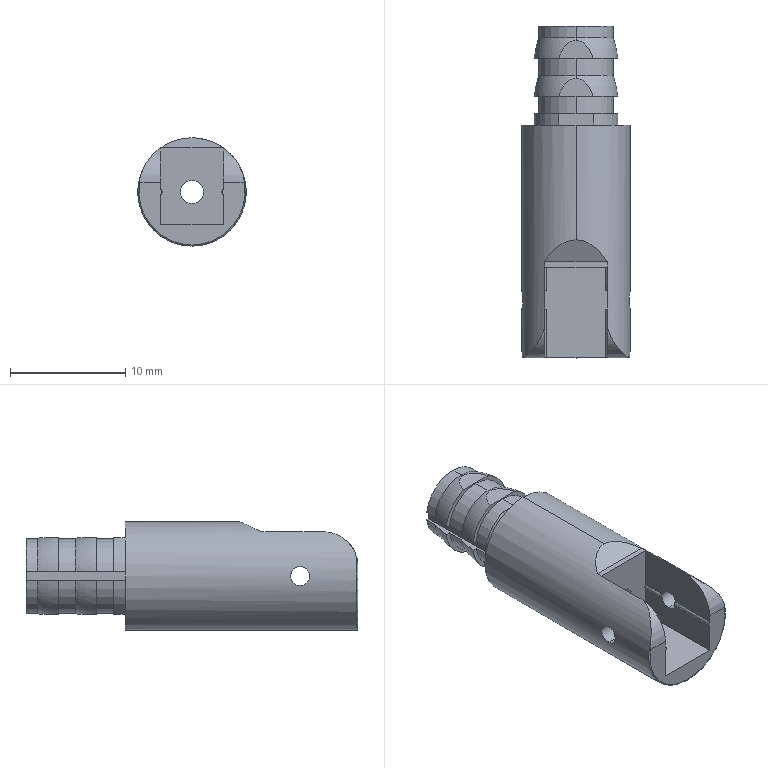Part | SolidWorks | features ICE 6, Fillet 1, Revolution 1 | 1 solid | 69 faces | box 9.4 x 28.8 x 9.4 mm | volume 935.936 mm3 | plane 30 | cylinder 29 | torus 10 | commonest cylinder face diameters 6.5 x9 0.445 x4 1.65 x4 7.3 x4 2 x2 5.35 x2